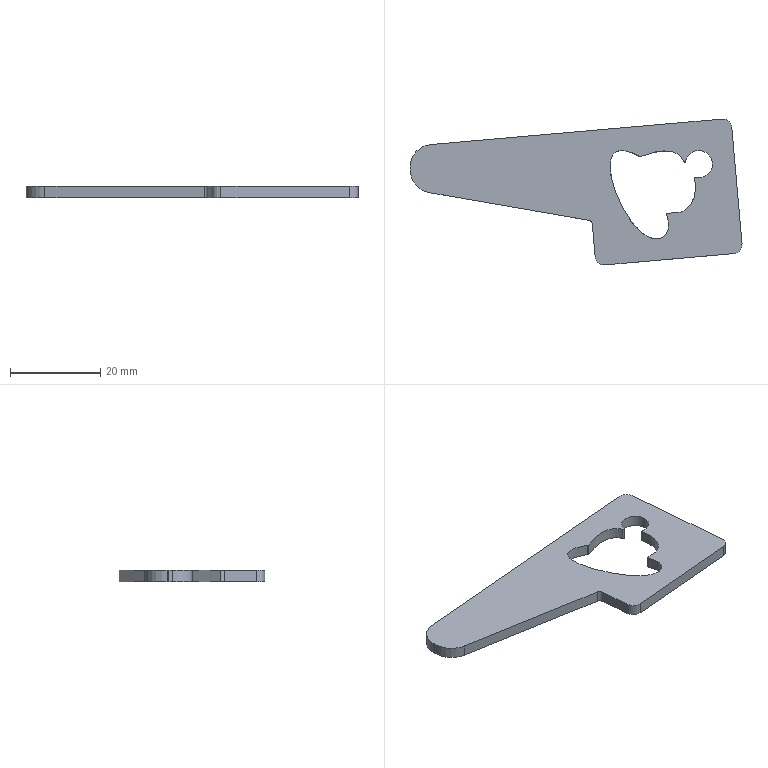Part | SolidWorks | features BaseBody 1 | 1 solid | 28 faces | box 73.757 x 32.407 x 2.5 mm | volume 3155 mm3 | cylinder 16 | plane 9 | spline 3 | commonest cylinder face diameters 0.4 x6 4 x3 6 x3 10 x3 2 x1
STEP:
#1=CARTESIAN_POINT('',(11.35,-18.25,15.));
#2=VERTEX_POINT('',#1);
#3=CARTESIAN_POINT('',(5.409,-17.656,15.));
#4=VERTEX_POINT('',#3);
#5=CARTESIAN_POINT('',(8.35,-18.25,15.));
#6=DIRECTION('',(0.,0.,1.));
#7=DIRECTION('',(1.,0.,0.));
#8=AXIS2_PLACEMENT_3D('',#5,#6,#7);
#9=CIRCLE('',#8,3.);
#10=EDGE_CURVE('',#2,#4,#9,.T.);
#11=ORIENTED_EDGE('',*,*,#10,.F.);
#12=CARTESIAN_POINT('',(11.35,-18.25,17.5));
#13=VERTEX_POINT('',#12);
#14=CARTESIAN_POINT('',(11.35,-18.25,15.));
#15=DIRECTION('',(0.,0.,1.));
#16=VECTOR('',#15,1000.);
#17=LINE('',#14,#16);
#18=EDGE_CURVE('',#2,#13,#17,.T.);
#19=ORIENTED_EDGE('',*,*,#18,.T.);
#20=CARTESIAN_POINT('',(5.409,-17.656,17.5));
#21=VERTEX_POINT('',#20);
#22=CARTESIAN_POINT('',(8.35,-18.25,17.5));
#23=DIRECTION('',(0.,0.,-1.));
#24=DIRECTION('',(1.,0.,0.));
#25=AXIS2_PLACEMENT_3D('',#22,#23,#24);
#26=CIRCLE('',#25,3.);
#27=EDGE_CURVE('',#21,#13,#26,.T.);
#28=ORIENTED_EDGE('',*,*,#27,.F.);
#29=CARTESIAN_POINT('',(5.409,-17.656,15.));
#30=DIRECTION('',(0.,0.,1.));
#31=VECTOR('',#30,1000.);
#32=LINE('',#29,#31);
#33=EDGE_CURVE('',#4,#21,#32,.T.);
#34=ORIENTED_EDGE('',*,*,#33,.F.);
#35=EDGE_LOOP('',(#11,#19,#28,#34));
#36=FACE_OUTER_BOUND('',#35,.T.);
#37=CARTESIAN_POINT('',(8.35,-18.25,15.));
#38=DIRECTION('',(0.,0.,1.));
#39=DIRECTION('',(1.,0.,0.));
#40=AXIS2_PLACEMENT_3D('',#37,#38,#39);
#41=CYLINDRICAL_SURFACE('',#40,3.);
#42=ADVANCED_FACE('',(#36),#41,.F.);
#43=CARTESIAN_POINT('',(-55.818,-18.909,17.5));
#44=VERTEX_POINT('',#43);
#45=CARTESIAN_POINT('',(-55.799,-19.345,17.5));
#46=VERTEX_POINT('',#45);
#47=CARTESIAN_POINT('',(-50.818,-18.909,17.5));
#48=DIRECTION('',(0.,0.,1.));
#49=DIRECTION('',(-1.,0.,0.));
#50=AXIS2_PLACEMENT_3D('',#47,#48,#49);
#51=CIRCLE('',#50,5.);
#52=EDGE_CURVE('',#44,#46,#51,.T.);
#53=ORIENTED_EDGE('',*,*,#52,.F.);
#54=CARTESIAN_POINT('',(-55.818,-18.909,15.));
#55=VERTEX_POINT('',#54);
#56=CARTESIAN_POINT('',(-55.818,-18.909,23.765));
#57=DIRECTION('',(0.,0.,-1.));
#58=VECTOR('',#57,1000.);
#59=LINE('',#56,#58);
#60=EDGE_CURVE('',#44,#55,#59,.T.);
#61=ORIENTED_EDGE('',*,*,#60,.T.);
#62=CARTESIAN_POINT('',(-55.799,-19.345,15.));
#63=VERTEX_POINT('',#62);
#64=CARTESIAN_POINT('',(-50.818,-18.909,15.));
#65=DIRECTION('',(0.,0.,1.));
#66=DIRECTION('',(-1.,0.,0.));
#67=AXIS2_PLACEMENT_3D('',#64,#65,#66);
#68=CIRCLE('',#67,5.);
#69=EDGE_CURVE('',#55,#63,#68,.T.);
#70=ORIENTED_EDGE('',*,*,#69,.T.);
#71=CARTESIAN_POINT('',(-55.799,-19.345,23.765));
#72=DIRECTION('',(0.,0.,1.));
#73=VECTOR('',#72,1000.);
#74=LINE('',#71,#73);
#75=EDGE_CURVE('',#63,#46,#74,.T.);
#76=ORIENTED_EDGE('',*,*,#75,.T.);
#77=EDGE_LOOP('',(#53,#61,#70,#76));
#78=FACE_OUTER_BOUND('',#77,.T.);
#79=CARTESIAN_POINT('',(-50.818,-18.909,23.765));
#80=DIRECTION('',(0.,0.,-1.));
#81=DIRECTION('',(-1.,0.,0.));
#82=AXIS2_PLACEMENT_3D('',#79,#80,#81);
#83=CYLINDRICAL_SURFACE('',#82,5.);
#84=ADVANCED_FACE('',(#78),#83,.T.);
#85=CARTESIAN_POINT('',(1.217,-29.458,17.5));
#86=VERTEX_POINT('',#85);
#87=CARTESIAN_POINT('',(1.208,-29.397,17.5));
#88=VERTEX_POINT('',#87);
#89=CARTESIAN_POINT('',(1.408,-29.397,17.5));
#90=DIRECTION('',(0.,0.,-1.));
#91=DIRECTION('',(-1.,0.,0.));
#92=AXIS2_PLACEMENT_3D('',#89,#90,#91);
#93=CIRCLE('',#92,0.2);
#94=EDGE_CURVE('',#86,#88,#93,.T.);
#95=ORIENTED_EDGE('',*,*,#94,.T.);
#96=CARTESIAN_POINT('',(1.208,-29.397,15.));
#97=VERTEX_POINT('',#96);
#98=CARTESIAN_POINT('',(1.208,-29.397,20.759));
#99=DIRECTION('',(0.,0.,-1.));
#100=VECTOR('',#99,1000.);
#101=LINE('',#98,#100);
#102=EDGE_CURVE('',#88,#97,#101,.T.);
#103=ORIENTED_EDGE('',*,*,#102,.T.);
#104=CARTESIAN_POINT('',(1.217,-29.458,15.));
#105=VERTEX_POINT('',#104);
#106=CARTESIAN_POINT('',(1.408,-29.397,15.));
#107=DIRECTION('',(0.,0.,1.));
#108=DIRECTION('',(-1.,0.,0.));
#109=AXIS2_PLACEMENT_3D('',#106,#107,#108);
#110=CIRCLE('',#109,0.2);
#111=EDGE_CURVE('',#97,#105,#110,.T.);
#112=ORIENTED_EDGE('',*,*,#111,.T.);
#113=CARTESIAN_POINT('',(1.217,-29.458,16.25));
#114=DIRECTION('',(0.,0.,1.));
#115=VECTOR('',#114,1000.);
#116=LINE('',#113,#115);
#117=EDGE_CURVE('',#105,#86,#116,.T.);
#118=ORIENTED_EDGE('',*,*,#117,.T.);
#119=EDGE_LOOP('',(#95,#103,#112,#118));
#120=FACE_OUTER_BOUND('',#119,.T.);
#121=CARTESIAN_POINT('',(1.408,-29.397,20.759));
#122=DIRECTION('',(0.,0.,-1.));
#123=DIRECTION('',(-1.,0.,0.));
#124=AXIS2_PLACEMENT_3D('',#121,#122,#123);
#125=CYLINDRICAL_SURFACE('',#124,0.2);
#126=ADVANCED_FACE('',(#120),#125,.T.);
#127=CARTESIAN_POINT('',(7.403,-21.403,17.5));
#128=VERTEX_POINT('',#127);
#129=CARTESIAN_POINT('',(7.398,-21.36,17.5));
#130=VERTEX_POINT('',#129);
#131=CARTESIAN_POINT('',(7.598,-21.36,17.5));
#132=DIRECTION('',(0.,0.,-1.));
#133=DIRECTION('',(-1.,0.,0.));
#134=AXIS2_PLACEMENT_3D('',#131,#132,#133);
#135=CIRCLE('',#134,0.2);
#136=EDGE_CURVE('',#128,#130,#135,.T.);
#137=ORIENTED_EDGE('',*,*,#136,.T.);
#138=CARTESIAN_POINT('',(7.398,-21.36,15.));
#139=VERTEX_POINT('',#138);
#140=CARTESIAN_POINT('',(7.398,-21.36,20.759));
#141=DIRECTION('',(0.,0.,-1.));
#142=VECTOR('',#141,1000.);
#143=LINE('',#140,#142);
#144=EDGE_CURVE('',#130,#139,#143,.T.);
#145=ORIENTED_EDGE('',*,*,#144,.T.);
#146=CARTESIAN_POINT('',(7.403,-21.403,15.));
#147=VERTEX_POINT('',#146);
#148=CARTESIAN_POINT('',(7.598,-21.36,15.));
#149=DIRECTION('',(0.,0.,1.));
#150=DIRECTION('',(-1.,0.,0.));
#151=AXIS2_PLACEMENT_3D('',#148,#149,#150);
#152=CIRCLE('',#151,0.2);
#153=EDGE_CURVE('',#139,#147,#152,.T.);
#154=ORIENTED_EDGE('',*,*,#153,.T.);
#155=CARTESIAN_POINT('',(7.403,-21.403,16.25));
#156=DIRECTION('',(0.,0.,1.));
#157=VECTOR('',#156,1000.);
#158=LINE('',#155,#157);
#159=EDGE_CURVE('',#147,#128,#158,.T.);
#160=ORIENTED_EDGE('',*,*,#159,.T.);
#161=EDGE_LOOP('',(#137,#145,#154,#160));
#162=FACE_OUTER_BOUND('',#161,.T.);
#163=CARTESIAN_POINT('',(7.598,-21.36,20.759));
#164=DIRECTION('',(0.,0.,-1.));
#165=DIRECTION('',(-1.,0.,0.));
#166=AXIS2_PLACEMENT_3D('',#163,#164,#165);
#167=CYLINDRICAL_SURFACE('',#166,0.2);
#168=ADVANCED_FACE('',(#162),#167,.T.);
#169=CARTESIAN_POINT('',(5.629,-28.182,17.5));
#170=VERTEX_POINT('',#169);
#171=CARTESIAN_POINT('',(3.837,-28.984,17.5));
#172=VERTEX_POINT('',#171);
#173=CARTESIAN_POINT('',(3.575,-25.996,17.5));
#174=DIRECTION('',(0.,0.,-1.));
#175=DIRECTION('',(1.,0.,0.));
#176=AXIS2_PLACEMENT_3D('',#173,#174,#175);
#177=CIRCLE('',#176,3.);
#178=EDGE_CURVE('',#170,#172,#177,.T.);
#179=ORIENTED_EDGE('',*,*,#178,.T.);
#180=CARTESIAN_POINT('',(1.39,-29.198,17.5));
#181=VERTEX_POINT('',#180);
#182=CARTESIAN_POINT('',(3.837,-28.984,17.5));
#183=DIRECTION('',(-0.9962,-0.08716,0.));
#184=VECTOR('',#183,1000.);
#185=LINE('',#182,#184);
#186=EDGE_CURVE('',#172,#181,#185,.T.);
#187=ORIENTED_EDGE('',*,*,#186,.T.);
#188=CARTESIAN_POINT('',(1.408,-29.397,17.5));
#189=DIRECTION('',(0.,0.,-1.));
#190=DIRECTION('',(-1.,0.,0.));
#191=AXIS2_PLACEMENT_3D('',#188,#189,#190);
#192=CIRCLE('',#191,0.2);
#193=EDGE_CURVE('',#88,#181,#192,.T.);
#194=ORIENTED_EDGE('',*,*,#193,.F.);
#195=ORIENTED_EDGE('',*,*,#94,.F.);
#196=CARTESIAN_POINT('',(-4.863,-16.57,17.5));
#197=VERTEX_POINT('',#196);
#198=CARTESIAN_POINT('',(1.217,-29.458,17.5));
#199=CARTESIAN_POINT('',(2.365,-33.062,17.5));
#200=CARTESIAN_POINT('',(-1.868,-37.339,17.5));
#201=CARTESIAN_POINT('',(-10.191,-27.786,17.5));
#202=CARTESIAN_POINT('',(-12.869,-14.51,17.5));
#203=CARTESIAN_POINT('',(-7.281,-15.123,17.5));
#204=CARTESIAN_POINT('',(-4.863,-16.57,17.5));
#205=B_SPLINE_CURVE_WITH_KNOTS('',3,(#198,#199,#200,#201,#202,#203,#204),.UNSPECIFIED.,.F.,.F.,(4,1,1,1,4),(0.,0.006113,0.01872,0.03058,0.03634),.UNSPECIFIED.);
#206=EDGE_CURVE('',#86,#197,#205,.T.);
#207=ORIENTED_EDGE('',*,*,#206,.T.);
#208=CARTESIAN_POINT('',(-4.693,-16.587,17.5));
#209=VERTEX_POINT('',#208);
#210=CARTESIAN_POINT('',(-4.76,-16.398,17.5));
#211=DIRECTION('',(0.,0.,-1.));
#212=DIRECTION('',(-1.,0.,0.));
#213=AXIS2_PLACEMENT_3D('',#210,#211,#212);
#214=CIRCLE('',#213,0.2);
#215=EDGE_CURVE('',#209,#197,#214,.T.);
#216=ORIENTED_EDGE('',*,*,#215,.F.);
#217=CARTESIAN_POINT('',(5.033,-17.703,17.5));
#218=VERTEX_POINT('',#217);
#219=CARTESIAN_POINT('',(-4.693,-16.587,17.5));
#220=CARTESIAN_POINT('',(-1.674,-15.514,17.5));
#221=CARTESIAN_POINT('',(2.462,-14.423,17.5));
#222=CARTESIAN_POINT('',(4.678,-16.963,17.5));
#223=CARTESIAN_POINT('',(5.033,-17.703,17.5));
#224=B_SPLINE_CURVE_WITH_KNOTS('',3,(#219,#220,#221,#222,#223),.UNSPECIFIED.,.F.,.F.,(4,1,4),(0.,0.008476,0.01075),.UNSPECIFIED.);
#225=EDGE_CURVE('',#209,#218,#224,.T.);
#226=ORIENTED_EDGE('',*,*,#225,.T.);
#227=CARTESIAN_POINT('',(5.213,-17.617,17.5));
#228=DIRECTION('',(0.,0.,-1.));
#229=DIRECTION('',(-1.,0.,0.));
#230=AXIS2_PLACEMENT_3D('',#227,#228,#229);
#231=CIRCLE('',#230,0.2);
#232=EDGE_CURVE('',#21,#218,#231,.T.);
#233=ORIENTED_EDGE('',*,*,#232,.F.);
#234=ORIENTED_EDGE('',*,*,#27,.T.);
#235=CARTESIAN_POINT('',(7.645,-21.166,17.5));
#236=VERTEX_POINT('',#235);
#237=CARTESIAN_POINT('',(8.35,-18.25,17.5));
#238=DIRECTION('',(0.,0.,-1.));
#239=DIRECTION('',(1.,0.,0.));
#240=AXIS2_PLACEMENT_3D('',#237,#238,#239);
#241=CIRCLE('',#240,3.);
#242=EDGE_CURVE('',#13,#236,#241,.T.);
#243=ORIENTED_EDGE('',*,*,#242,.T.);
#244=CARTESIAN_POINT('',(7.598,-21.36,17.5));
#245=DIRECTION('',(0.,0.,-1.));
#246=DIRECTION('',(-1.,0.,0.));
#247=AXIS2_PLACEMENT_3D('',#244,#245,#246);
#248=CIRCLE('',#247,0.2);
#249=EDGE_CURVE('',#130,#236,#248,.T.);
#250=ORIENTED_EDGE('',*,*,#249,.F.);
#251=ORIENTED_EDGE('',*,*,#136,.F.);
#252=CARTESIAN_POINT('',(7.403,-21.403,17.5));
#253=CARTESIAN_POINT('',(8.013,-24.239,17.5));
#254=CARTESIAN_POINT('',(7.422,-26.499,17.5));
#255=CARTESIAN_POINT('',(5.629,-28.182,17.5));
#256=B_SPLINE_CURVE_WITH_KNOTS('',3,(#252,#253,#254,#255),.UNSPECIFIED.,.F.,.F.,(4,4),(0.,1.),.UNSPECIFIED.);
#257=EDGE_CURVE('',#128,#170,#256,.T.);
#258=ORIENTED_EDGE('',*,*,#257,.T.);
#259=EDGE_LOOP('',(#179,#187,#194,#195,#207,#216,#226,#233,#234,#243,#250,#251,#258));
#260=FACE_BOUND('',#259,.T.);
#261=CARTESIAN_POINT('',(-12.527,-40.655,17.5));
#262=VERTEX_POINT('',#261);
#263=CARTESIAN_POINT('',(16.114,-38.149,17.5));
#264=VERTEX_POINT('',#263);
#265=CARTESIAN_POINT('',(-12.527,-40.655,17.5));
#266=DIRECTION('',(0.9962,0.08716,0.));
#267=VECTOR('',#266,1000.);
#268=LINE('',#265,#267);
#269=EDGE_CURVE('',#262,#264,#268,.T.);
#270=ORIENTED_EDGE('',*,*,#269,.T.);
#271=CARTESIAN_POINT('',(17.932,-35.982,17.5));
#272=VERTEX_POINT('',#271);
#273=CARTESIAN_POINT('',(15.94,-36.157,17.5));
#274=DIRECTION('',(0.,0.,1.));
#275=DIRECTION('',(-1.,0.,0.));
#276=AXIS2_PLACEMENT_3D('',#273,#274,#275);
#277=CIRCLE('',#276,2.);
#278=EDGE_CURVE('',#264,#272,#277,.T.);
#279=ORIENTED_EDGE('',*,*,#278,.T.);
#280=CARTESIAN_POINT('',(15.666,-10.081,17.5));
#281=VERTEX_POINT('',#280);
#282=CARTESIAN_POINT('',(17.932,-35.982,17.5));
#283=DIRECTION('',(-0.08716,0.9962,0.));
#284=VECTOR('',#283,1000.);
#285=LINE('',#282,#284);
#286=EDGE_CURVE('',#272,#281,#285,.T.);
#287=ORIENTED_EDGE('',*,*,#286,.T.);
#288=CARTESIAN_POINT('',(13.499,-8.263,17.5));
#289=VERTEX_POINT('',#288);
#290=CARTESIAN_POINT('',(13.674,-10.256,17.5));
#291=DIRECTION('',(0.,0.,1.));
#292=DIRECTION('',(-1.,0.,0.));
#293=AXIS2_PLACEMENT_3D('',#290,#291,#292);
#294=CIRCLE('',#293,2.);
#295=EDGE_CURVE('',#281,#289,#294,.T.);
#296=ORIENTED_EDGE('',*,*,#295,.T.);
#297=CARTESIAN_POINT('',(-51.253,-13.928,17.5));
#298=VERTEX_POINT('',#297);
#299=CARTESIAN_POINT('',(13.499,-8.263,17.5));
#300=DIRECTION('',(-0.9962,-0.08716,0.));
#301=VECTOR('',#300,1000.);
#302=LINE('',#299,#301);
#303=EDGE_CURVE('',#289,#298,#302,.T.);
#304=ORIENTED_EDGE('',*,*,#303,.T.);
#305=CARTESIAN_POINT('',(-50.818,-18.909,17.5));
#306=DIRECTION('',(0.,0.,1.));
#307=DIRECTION('',(-1.,0.,0.));
#308=AXIS2_PLACEMENT_3D('',#305,#306,#307);
#309=CIRCLE('',#308,5.);
#310=EDGE_CURVE('',#298,#44,#309,.T.);
#311=ORIENTED_EDGE('',*,*,#310,.T.);
#312=ORIENTED_EDGE('',*,*,#52,.T.);
#313=CARTESIAN_POINT('',(-55.733,-20.095,17.5));
#314=VERTEX_POINT('',#313);
#315=CARTESIAN_POINT('',(-56.234,-14.364,17.5));
#316=DIRECTION('',(-0.08716,0.9962,0.));
#317=VECTOR('',#316,1000.);
#318=LINE('',#315,#317);
#319=EDGE_CURVE('',#314,#46,#318,.T.);
#320=ORIENTED_EDGE('',*,*,#319,.F.);
#321=CARTESIAN_POINT('',(-51.607,-24.585,17.5));
#322=VERTEX_POINT('',#321);
#323=CARTESIAN_POINT('',(-50.752,-19.659,17.5));
#324=DIRECTION('',(0.,0.,1.));
#325=DIRECTION('',(-1.,0.,0.));
#326=AXIS2_PLACEMENT_3D('',#323,#324,#325);
#327=CIRCLE('',#326,5.);
#328=EDGE_CURVE('',#314,#322,#327,.T.);
#329=ORIENTED_EDGE('',*,*,#328,.T.);
#330=CARTESIAN_POINT('',(-16.149,-30.736,17.5));
#331=VERTEX_POINT('',#330);
#332=CARTESIAN_POINT('',(-51.607,-24.585,17.5));
#333=DIRECTION('',(0.9853,-0.1709,0.));
#334=VECTOR('',#333,1000.);
#335=LINE('',#332,#334);
#336=EDGE_CURVE('',#322,#331,#335,.T.);
#337=ORIENTED_EDGE('',*,*,#336,.T.);
#338=CARTESIAN_POINT('',(-15.324,-31.634,17.5));
#339=VERTEX_POINT('',#338);
#340=CARTESIAN_POINT('',(-16.32,-31.721,17.5));
#341=DIRECTION('',(0.,0.,-1.));
#342=DIRECTION('',(1.,0.,0.));
#343=AXIS2_PLACEMENT_3D('',#340,#341,#342);
#344=CIRCLE('',#343,1.);
#345=EDGE_CURVE('',#331,#339,#344,.T.);
#346=ORIENTED_EDGE('',*,*,#345,.T.);
#347=CARTESIAN_POINT('',(-14.693,-38.837,17.5));
#348=VERTEX_POINT('',#347);
#349=CARTESIAN_POINT('',(-15.324,-31.634,17.5));
#350=DIRECTION('',(0.08716,-0.9962,0.));
#351=VECTOR('',#350,1000.);
#352=LINE('',#349,#351);
#353=EDGE_CURVE('',#339,#348,#352,.T.);
#354=ORIENTED_EDGE('',*,*,#353,.T.);
#355=CARTESIAN_POINT('',(-12.701,-38.662,17.5));
#356=DIRECTION('',(0.,0.,1.));
#357=DIRECTION('',(-1.,0.,0.));
#358=AXIS2_PLACEMENT_3D('',#355,#356,#357);
#359=CIRCLE('',#358,2.);
#360=EDGE_CURVE('',#348,#262,#359,.T.);
#361=ORIENTED_EDGE('',*,*,#360,.T.);
#362=EDGE_LOOP('',(#270,#279,#287,#296,#304,#311,#312,#320,#329,#337,#346,#354,#361));
#363=FACE_OUTER_BOUND('',#362,.T.);
#364=CARTESIAN_POINT('',(15.492,-8.089,17.5));
#365=DIRECTION('',(0.,0.,1.));
#366=DIRECTION('',(1.,0.,0.));
#367=AXIS2_PLACEMENT_3D('',#364,#365,#366);
#368=PLANE('',#367);
#369=ADVANCED_FACE('',(#260,#363),#368,.T.);
#370=ORIENTED_EDGE('',*,*,#186,.F.);
#371=CARTESIAN_POINT('',(3.837,-28.984,15.));
#372=VERTEX_POINT('',#371);
#373=CARTESIAN_POINT('',(3.837,-28.984,15.));
#374=DIRECTION('',(0.,0.,-1.));
#375=VECTOR('',#374,1000.);
#376=LINE('',#373,#375);
#377=EDGE_CURVE('',#172,#372,#376,.T.);
#378=ORIENTED_EDGE('',*,*,#377,.T.);
#379=CARTESIAN_POINT('',(1.39,-29.198,15.));
#380=VERTEX_POINT('',#379);
#381=CARTESIAN_POINT('',(4.735,-28.906,15.));
#382=DIRECTION('',(-0.9962,-0.08716,0.));
#383=VECTOR('',#382,1000.);
#384=LINE('',#381,#383);
#385=EDGE_CURVE('',#372,#380,#384,.T.);
#386=ORIENTED_EDGE('',*,*,#385,.T.);
#387=CARTESIAN_POINT('',(1.39,-29.198,15.));
#388=DIRECTION('',(0.,0.,1.));
#389=VECTOR('',#388,1000.);
#390=LINE('',#387,#389);
#391=EDGE_CURVE('',#380,#181,#390,.T.);
#392=ORIENTED_EDGE('',*,*,#391,.T.);
#393=EDGE_LOOP('',(#370,#378,#386,#392));
#394=FACE_OUTER_BOUND('',#393,.T.);
#395=CARTESIAN_POINT('',(4.735,-28.906,15.));
#396=DIRECTION('',(-0.08716,0.9962,0.));
#397=DIRECTION('',(-0.9962,-0.08716,0.));
#398=AXIS2_PLACEMENT_3D('',#395,#396,#397);
#399=PLANE('',#398);
#400=ADVANCED_FACE('',(#394),#399,.T.);
#401=CARTESIAN_POINT('',(5.629,-28.182,15.));
#402=VERTEX_POINT('',#401);
#403=CARTESIAN_POINT('',(5.629,-28.182,11.14));
#404=DIRECTION('',(0.,0.,1.));
#405=VECTOR('',#404,1000.);
#406=LINE('',#403,#405);
#407=EDGE_CURVE('',#402,#170,#406,.T.);
#408=ORIENTED_EDGE('',*,*,#407,.F.);
#409=CARTESIAN_POINT('',(3.575,-25.996,15.));
#410=DIRECTION('',(0.,0.,1.));
#411=DIRECTION('',(1.,0.,0.));
#412=AXIS2_PLACEMENT_3D('',#409,#410,#411);
#413=CIRCLE('',#412,3.);
#414=EDGE_CURVE('',#372,#402,#413,.T.);
#415=ORIENTED_EDGE('',*,*,#414,.F.);
#416=ORIENTED_EDGE('',*,*,#377,.F.);
#417=ORIENTED_EDGE('',*,*,#178,.F.);
#418=EDGE_LOOP('',(#408,#415,#416,#417));
#419=FACE_OUTER_BOUND('',#418,.T.);
#420=CARTESIAN_POINT('',(3.575,-25.996,11.14));
#421=DIRECTION('',(0.,0.,1.));
#422=DIRECTION('',(1.,0.,0.));
#423=AXIS2_PLACEMENT_3D('',#420,#421,#422);
#424=CYLINDRICAL_SURFACE('',#423,3.);
#425=ADVANCED_FACE('',(#419),#424,.F.);
#426=ORIENTED_EDGE('',*,*,#159,.F.);
#427=CARTESIAN_POINT('',(5.629,-28.182,15.));
#428=CARTESIAN_POINT('',(7.422,-26.499,15.));
#429=CARTESIAN_POINT('',(8.013,-24.239,15.));
#430=CARTESIAN_POINT('',(7.403,-21.403,15.));
#431=B_SPLINE_CURVE_WITH_KNOTS('',3,(#427,#428,#429,#430),.UNSPECIFIED.,.F.,.F.,(4,4),(0.,1.),.UNSPECIFIED.);
#432=EDGE_CURVE('',#402,#147,#431,.T.);
#433=ORIENTED_EDGE('',*,*,#432,.F.);
#434=ORIENTED_EDGE('',*,*,#407,.T.);
#435=ORIENTED_EDGE('',*,*,#257,.F.);
#436=EDGE_LOOP('',(#426,#433,#434,#435));
#437=FACE_OUTER_BOUND('',#436,.T.);
#438=CARTESIAN_POINT('',(5.629,-28.182,15.));
#439=CARTESIAN_POINT('',(5.629,-28.182,17.5));
#440=CARTESIAN_POINT('',(6.029,-27.807,15.));
#441=CARTESIAN_POINT('',(6.029,-27.807,17.5));
#442=CARTESIAN_POINT('',(7.554,-25.995,15.));
#443=CARTESIAN_POINT('',(7.554,-25.995,17.5));
#444=CARTESIAN_POINT('',(7.877,-23.607,15.));
#445=CARTESIAN_POINT('',(7.877,-23.607,17.5));
#446=CARTESIAN_POINT('',(7.403,-21.403,15.));
#447=CARTESIAN_POINT('',(7.403,-21.403,17.5));
#448=B_SPLINE_SURFACE_WITH_KNOTS('',3,1,((#438,#439),(#440,#441),(#442,#443),(#444,#445),(#446,#447)),.UNSPECIFIED.,.F.,.F.,.F.,(4,1,4),(2,2),(0.009234,0.2282,0.9918),(0.,1.),.UNSPECIFIED.);
#449=ADVANCED_FACE('',(#437),#448,.F.);
#450=ORIENTED_EDGE('',*,*,#18,.F.);
#451=CARTESIAN_POINT('',(7.645,-21.166,15.));
#452=VERTEX_POINT('',#451);
#453=CARTESIAN_POINT('',(8.35,-18.25,15.));
#454=DIRECTION('',(0.,0.,1.));
#455=DIRECTION('',(1.,0.,0.));
#456=AXIS2_PLACEMENT_3D('',#453,#454,#455);
#457=CIRCLE('',#456,3.);
#458=EDGE_CURVE('',#452,#2,#457,.T.);
#459=ORIENTED_EDGE('',*,*,#458,.F.);
#460=CARTESIAN_POINT('',(7.645,-21.166,15.));
#461=DIRECTION('',(0.,0.,-1.));
#462=VECTOR('',#461,1000.);
#463=LINE('',#460,#462);
#464=EDGE_CURVE('',#236,#452,#463,.T.);
#465=ORIENTED_EDGE('',*,*,#464,.F.);
#466=ORIENTED_EDGE('',*,*,#242,.F.);
#467=EDGE_LOOP('',(#450,#459,#465,#466));
#468=FACE_OUTER_BOUND('',#467,.T.);
#469=CARTESIAN_POINT('',(8.35,-18.25,15.));
#470=DIRECTION('',(0.,0.,1.));
#471=DIRECTION('',(1.,0.,0.));
#472=AXIS2_PLACEMENT_3D('',#469,#470,#471);
#473=CYLINDRICAL_SURFACE('',#472,3.);
#474=ADVANCED_FACE('',(#468),#473,.F.);
#475=CARTESIAN_POINT('',(-4.693,-16.587,15.));
#476=VERTEX_POINT('',#475);
#477=CARTESIAN_POINT('',(-4.693,-16.587,16.25));
#478=DIRECTION('',(0.,0.,1.));
#479=VECTOR('',#478,1000.);
#480=LINE('',#477,#479);
#481=EDGE_CURVE('',#476,#209,#480,.T.);
#482=ORIENTED_EDGE('',*,*,#481,.F.);
#483=CARTESIAN_POINT('',(5.033,-17.703,15.));
#484=VERTEX_POINT('',#483);
#485=CARTESIAN_POINT('',(5.033,-17.703,15.));
#486=CARTESIAN_POINT('',(4.678,-16.963,15.));
#487=CARTESIAN_POINT('',(2.462,-14.423,15.));
#488=CARTESIAN_POINT('',(-1.674,-15.514,15.));
#489=CARTESIAN_POINT('',(-4.693,-16.587,15.));
#490=B_SPLINE_CURVE_WITH_KNOTS('',3,(#485,#486,#487,#488,#489),.UNSPECIFIED.,.F.,.F.,(4,1,4),(0.,0.002298,0.01085),.UNSPECIFIED.);
#491=EDGE_CURVE('',#484,#476,#490,.T.);
#492=ORIENTED_EDGE('',*,*,#491,.F.);
#493=CARTESIAN_POINT('',(5.033,-17.703,16.25));
#494=DIRECTION('',(0.,0.,-1.));
#495=VECTOR('',#494,1000.);
#496=LINE('',#493,#495);
#497=EDGE_CURVE('',#218,#484,#496,.T.);
#498=ORIENTED_EDGE('',*,*,#497,.F.);
#499=ORIENTED_EDGE('',*,*,#225,.F.);
#500=EDGE_LOOP('',(#482,#492,#498,#499));
#501=FACE_OUTER_BOUND('',#500,.T.);
#502=CARTESIAN_POINT('',(5.033,-17.703,15.));
#503=CARTESIAN_POINT('',(5.033,-17.703,17.5));
#504=CARTESIAN_POINT('',(4.678,-16.963,15.));
#505=CARTESIAN_POINT('',(4.678,-16.963,17.5));
#506=CARTESIAN_POINT('',(2.462,-14.423,15.));
#507=CARTESIAN_POINT('',(2.462,-14.423,17.5));
#508=CARTESIAN_POINT('',(-1.674,-15.514,15.));
#509=CARTESIAN_POINT('',(-1.674,-15.514,17.5));
#510=CARTESIAN_POINT('',(-4.693,-16.587,15.));
#511=CARTESIAN_POINT('',(-4.693,-16.587,17.5));
#512=B_SPLINE_SURFACE_WITH_KNOTS('',3,1,((#502,#503),(#504,#505),(#506,#507),(#508,#509),(#510,#511)),.UNSPECIFIED.,.F.,.F.,.F.,(4,1,4),(2,2),(0.00811,0.2164,0.9912),(0.,1.),.UNSPECIFIED.);
#513=ADVANCED_FACE('',(#501),#512,.F.);
#514=ORIENTED_EDGE('',*,*,#117,.F.);
#515=CARTESIAN_POINT('',(-4.863,-16.57,15.));
#516=VERTEX_POINT('',#515);
#517=CARTESIAN_POINT('',(-4.863,-16.57,15.));
#518=CARTESIAN_POINT('',(-7.281,-15.123,15.));
#519=CARTESIAN_POINT('',(-12.869,-14.51,15.));
#520=CARTESIAN_POINT('',(-10.191,-27.786,15.));
#521=CARTESIAN_POINT('',(-1.868,-37.339,15.));
#522=CARTESIAN_POINT('',(2.365,-33.062,15.));
#523=CARTESIAN_POINT('',(1.217,-29.458,15.));
#524=B_SPLINE_CURVE_WITH_KNOTS('',3,(#517,#518,#519,#520,#521,#522,#523),.UNSPECIFIED.,.F.,.F.,(4,1,1,1,4),(0.,0.005774,0.01766,0.03028,0.03641),.UNSPECIFIED.);
#525=EDGE_CURVE('',#516,#105,#524,.T.);
#526=ORIENTED_EDGE('',*,*,#525,.F.);
#527=CARTESIAN_POINT('',(-4.863,-16.57,16.25));
#528=DIRECTION('',(0.,0.,-1.));
#529=VECTOR('',#528,1000.);
#530=LINE('',#527,#529);
#531=EDGE_CURVE('',#197,#516,#530,.T.);
#532=ORIENTED_EDGE('',*,*,#531,.F.);
#533=ORIENTED_EDGE('',*,*,#206,.F.);
#534=EDGE_LOOP('',(#514,#526,#532,#533));
#535=FACE_OUTER_BOUND('',#534,.T.);
#536=CARTESIAN_POINT('',(-4.863,-16.57,15.));
#537=CARTESIAN_POINT('',(-4.863,-16.57,17.5));
#538=CARTESIAN_POINT('',(-7.281,-15.123,15.));
#539=CARTESIAN_POINT('',(-7.281,-15.123,17.5));
#540=CARTESIAN_POINT('',(-12.869,-14.51,15.));
#541=CARTESIAN_POINT('',(-12.869,-14.51,17.5));
#542=CARTESIAN_POINT('',(-10.191,-27.786,15.));
#543=CARTESIAN_POINT('',(-10.191,-27.786,17.5));
#544=CARTESIAN_POINT('',(-1.868,-37.339,15.));
#545=CARTESIAN_POINT('',(-1.868,-37.339,17.5));
#546=CARTESIAN_POINT('',(2.365,-33.062,15.));
#547=CARTESIAN_POINT('',(2.365,-33.062,17.5));
#548=CARTESIAN_POINT('',(1.217,-29.458,15.));
#549=CARTESIAN_POINT('',(1.217,-29.458,17.5));
#550=B_SPLINE_SURFACE_WITH_KNOTS('',3,1,((#536,#537),(#538,#539),(#540,#541),(#542,#543),(#544,#545),(#546,#547),(#548,#549)),.UNSPECIFIED.,.F.,.F.,.F.,(4,1,1,1,4),(2,2),(0.006613,0.1633,0.4858,0.8285,0.9947),(0.,1.),.UNSPECIFIED.);
#551=ADVANCED_FACE('',(#535),#550,.F.);
#552=CARTESIAN_POINT('',(16.114,-38.149,15.));
#553=VERTEX_POINT('',#552);
#554=CARTESIAN_POINT('',(16.114,-38.149,20.759));
#555=DIRECTION('',(0.,0.,-1.));
#556=VECTOR('',#555,1000.);
#557=LINE('',#554,#556);
#558=EDGE_CURVE('',#264,#553,#557,.T.);
#559=ORIENTED_EDGE('',*,*,#558,.T.);
#560=CARTESIAN_POINT('',(17.932,-35.982,15.));
#561=VERTEX_POINT('',#560);
#562=CARTESIAN_POINT('',(15.94,-36.157,15.));
#563=DIRECTION('',(0.,0.,1.));
#564=DIRECTION('',(-1.,0.,0.));
#565=AXIS2_PLACEMENT_3D('',#562,#563,#564);
#566=CIRCLE('',#565,2.);
#567=EDGE_CURVE('',#553,#561,#566,.T.);
#568=ORIENTED_EDGE('',*,*,#567,.T.);
#569=CARTESIAN_POINT('',(17.932,-35.982,20.759));
#570=DIRECTION('',(0.,0.,1.));
#571=VECTOR('',#570,1000.);
#572=LINE('',#569,#571);
#573=EDGE_CURVE('',#561,#272,#572,.T.);
#574=ORIENTED_EDGE('',*,*,#573,.T.);
#575=ORIENTED_EDGE('',*,*,#278,.F.);
#576=EDGE_LOOP('',(#559,#568,#574,#575));
#577=FACE_OUTER_BOUND('',#576,.T.);
#578=CARTESIAN_POINT('',(15.94,-36.157,20.759));
#579=DIRECTION('',(0.,0.,-1.));
#580=DIRECTION('',(-1.,0.,0.));
#581=AXIS2_PLACEMENT_3D('',#578,#579,#580);
#582=CYLINDRICAL_SURFACE('',#581,2.);
#583=ADVANCED_FACE('',(#577),#582,.T.);
#584=CARTESIAN_POINT('',(-12.527,-40.655,15.));
#585=VERTEX_POINT('',#584);
#586=CARTESIAN_POINT('',(-14.519,-40.829,15.));
#587=DIRECTION('',(0.9962,0.08716,0.));
#588=VECTOR('',#587,1000.);
#589=LINE('',#586,#588);
#590=EDGE_CURVE('',#585,#553,#589,.T.);
#591=ORIENTED_EDGE('',*,*,#590,.T.);
#592=ORIENTED_EDGE('',*,*,#558,.F.);
#593=ORIENTED_EDGE('',*,*,#269,.F.);
#594=CARTESIAN_POINT('',(-12.527,-40.655,15.));
#595=DIRECTION('',(0.,0.,-1.));
#596=VECTOR('',#595,1000.);
#597=LINE('',#594,#596);
#598=EDGE_CURVE('',#262,#585,#597,.T.);
#599=ORIENTED_EDGE('',*,*,#598,.T.);
#600=EDGE_LOOP('',(#591,#592,#593,#599));
#601=FACE_OUTER_BOUND('',#600,.T.);
#602=CARTESIAN_POINT('',(-14.519,-40.829,15.));
#603=DIRECTION('',(0.08716,-0.9962,0.));
#604=DIRECTION('',(0.9962,0.08716,0.));
#605=AXIS2_PLACEMENT_3D('',#602,#603,#604);
#606=PLANE('',#605);
#607=ADVANCED_FACE('',(#601),#606,.T.);
#608=CARTESIAN_POINT('',(-14.693,-38.837,15.));
#609=VERTEX_POINT('',#608);
#610=CARTESIAN_POINT('',(-14.693,-38.837,20.759));
#611=DIRECTION('',(0.,0.,-1.));
#612=VECTOR('',#611,1000.);
#613=LINE('',#610,#612);
#614=EDGE_CURVE('',#348,#609,#613,.T.);
#615=ORIENTED_EDGE('',*,*,#614,.T.);
#616=CARTESIAN_POINT('',(-12.701,-38.662,15.));
#617=DIRECTION('',(0.,0.,1.));
#618=DIRECTION('',(-1.,0.,0.));
#619=AXIS2_PLACEMENT_3D('',#616,#617,#618);
#620=CIRCLE('',#619,2.);
#621=EDGE_CURVE('',#609,#585,#620,.T.);
#622=ORIENTED_EDGE('',*,*,#621,.T.);
#623=ORIENTED_EDGE('',*,*,#598,.F.);
#624=ORIENTED_EDGE('',*,*,#360,.F.);
#625=EDGE_LOOP('',(#615,#622,#623,#624));
#626=FACE_OUTER_BOUND('',#625,.T.);
#627=CARTESIAN_POINT('',(-12.701,-38.662,20.759));
#628=DIRECTION('',(0.,0.,-1.));
#629=DIRECTION('',(-1.,0.,0.));
#630=AXIS2_PLACEMENT_3D('',#627,#628,#629);
#631=CYLINDRICAL_SURFACE('',#630,2.);
#632=ADVANCED_FACE('',(#626),#631,.T.);
#633=CARTESIAN_POINT('',(-15.324,-31.634,15.));
#634=VERTEX_POINT('',#633);
#635=CARTESIAN_POINT('',(-15.391,-30.867,15.));
#636=DIRECTION('',(0.08716,-0.9962,0.));
#637=VECTOR('',#636,1000.);
#638=LINE('',#635,#637);
#639=EDGE_CURVE('',#634,#609,#638,.T.);
#640=ORIENTED_EDGE('',*,*,#639,.T.);
#641=ORIENTED_EDGE('',*,*,#614,.F.);
#642=ORIENTED_EDGE('',*,*,#353,.F.);
#643=CARTESIAN_POINT('',(-15.324,-31.634,15.));
#644=DIRECTION('',(0.,0.,-1.));
#645=VECTOR('',#644,1000.);
#646=LINE('',#643,#645);
#647=EDGE_CURVE('',#339,#634,#646,.T.);
#648=ORIENTED_EDGE('',*,*,#647,.T.);
#649=EDGE_LOOP('',(#640,#641,#642,#648));
#650=FACE_OUTER_BOUND('',#649,.T.);
#651=CARTESIAN_POINT('',(-15.391,-30.867,15.));
#652=DIRECTION('',(-0.9962,-0.08716,0.));
#653=DIRECTION('',(0.08716,-0.9962,0.));
#654=AXIS2_PLACEMENT_3D('',#651,#652,#653);
#655=PLANE('',#654);
#656=ADVANCED_FACE('',(#650),#655,.T.);
#657=ORIENTED_EDGE('',*,*,#336,.F.);
#658=CARTESIAN_POINT('',(-51.607,-24.585,15.));
#659=VERTEX_POINT('',#658);
#660=CARTESIAN_POINT('',(-51.607,-24.585,15.));
#661=DIRECTION('',(0.,0.,-1.));
#662=VECTOR('',#661,1000.);
#663=LINE('',#660,#662);
#664=EDGE_CURVE('',#322,#659,#663,.T.);
#665=ORIENTED_EDGE('',*,*,#664,.T.);
#666=CARTESIAN_POINT('',(-16.149,-30.736,15.));
#667=VERTEX_POINT('',#666);
#668=CARTESIAN_POINT('',(-55.398,-23.928,15.));
#669=DIRECTION('',(0.9853,-0.1709,0.));
#670=VECTOR('',#669,1000.);
#671=LINE('',#668,#670);
#672=EDGE_CURVE('',#659,#667,#671,.T.);
#673=ORIENTED_EDGE('',*,*,#672,.T.);
#674=CARTESIAN_POINT('',(-16.149,-30.736,15.));
#675=DIRECTION('',(0.,0.,1.));
#676=VECTOR('',#675,1000.);
#677=LINE('',#674,#676);
#678=EDGE_CURVE('',#667,#331,#677,.T.);
#679=ORIENTED_EDGE('',*,*,#678,.T.);
#680=EDGE_LOOP('',(#657,#665,#673,#679));
#681=FACE_OUTER_BOUND('',#680,.T.);
#682=CARTESIAN_POINT('',(-55.398,-23.928,15.));
#683=DIRECTION('',(-0.1709,-0.9853,0.));
#684=DIRECTION('',(0.9853,-0.1709,0.));
#685=AXIS2_PLACEMENT_3D('',#682,#683,#684);
#686=PLANE('',#685);
#687=ADVANCED_FACE('',(#681),#686,.T.);
#688=CARTESIAN_POINT('',(-55.733,-20.095,15.));
#689=VERTEX_POINT('',#688);
#690=CARTESIAN_POINT('',(-55.733,-20.095,23.765));
#691=DIRECTION('',(0.,0.,-1.));
#692=VECTOR('',#691,1000.);
#693=LINE('',#690,#692);
#694=EDGE_CURVE('',#314,#689,#693,.T.);
#695=ORIENTED_EDGE('',*,*,#694,.T.);
#696=CARTESIAN_POINT('',(-50.752,-19.659,15.));
#697=DIRECTION('',(0.,0.,1.));
#698=DIRECTION('',(-1.,0.,0.));
#699=AXIS2_PLACEMENT_3D('',#696,#697,#698);
#700=CIRCLE('',#699,5.);
#701=EDGE_CURVE('',#689,#659,#700,.T.);
#702=ORIENTED_EDGE('',*,*,#701,.T.);
#703=ORIENTED_EDGE('',*,*,#664,.F.);
#704=ORIENTED_EDGE('',*,*,#328,.F.);
#705=EDGE_LOOP('',(#695,#702,#703,#704));
#706=FACE_OUTER_BOUND('',#705,.T.);
#707=CARTESIAN_POINT('',(-50.752,-19.659,23.765));
#708=DIRECTION('',(0.,0.,-1.));
#709=DIRECTION('',(-1.,0.,0.));
#710=AXIS2_PLACEMENT_3D('',#707,#708,#709);
#711=CYLINDRICAL_SURFACE('',#710,5.);
#712=ADVANCED_FACE('',(#706),#711,.T.);
#713=ORIENTED_EDGE('',*,*,#60,.F.);
#714=ORIENTED_EDGE('',*,*,#310,.F.);
#715=CARTESIAN_POINT('',(-51.253,-13.928,15.));
#716=VERTEX_POINT('',#715);
#717=CARTESIAN_POINT('',(-51.253,-13.928,23.765));
#718=DIRECTION('',(0.,0.,-1.));
#719=VECTOR('',#718,1000.);
#720=LINE('',#717,#719);
#721=EDGE_CURVE('',#298,#716,#720,.T.);
#722=ORIENTED_EDGE('',*,*,#721,.T.);
#723=CARTESIAN_POINT('',(-50.818,-18.909,15.));
#724=DIRECTION('',(0.,0.,1.));
#725=DIRECTION('',(-1.,0.,0.));
#726=AXIS2_PLACEMENT_3D('',#723,#724,#725);
#727=CIRCLE('',#726,5.);
#728=EDGE_CURVE('',#716,#55,#727,.T.);
#729=ORIENTED_EDGE('',*,*,#728,.T.);
#730=EDGE_LOOP('',(#713,#714,#722,#729));
#731=FACE_OUTER_BOUND('',#730,.T.);
#732=CARTESIAN_POINT('',(-50.818,-18.909,23.765));
#733=DIRECTION('',(0.,0.,-1.));
#734=DIRECTION('',(-1.,0.,0.));
#735=AXIS2_PLACEMENT_3D('',#732,#733,#734);
#736=CYLINDRICAL_SURFACE('',#735,5.);
#737=ADVANCED_FACE('',(#731),#736,.T.);
#738=ORIENTED_EDGE('',*,*,#303,.F.);
#739=CARTESIAN_POINT('',(13.499,-8.263,15.));
#740=VERTEX_POINT('',#739);
#741=CARTESIAN_POINT('',(13.499,-8.263,15.));
#742=DIRECTION('',(0.,0.,-1.));
#743=VECTOR('',#742,1000.);
#744=LINE('',#741,#743);
#745=EDGE_CURVE('',#289,#740,#744,.T.);
#746=ORIENTED_EDGE('',*,*,#745,.T.);
#747=CARTESIAN_POINT('',(15.492,-8.089,15.));
#748=DIRECTION('',(-0.9962,-0.08716,0.));
#749=VECTOR('',#748,1000.);
#750=LINE('',#747,#749);
#751=EDGE_CURVE('',#740,#716,#750,.T.);
#752=ORIENTED_EDGE('',*,*,#751,.T.);
#753=ORIENTED_EDGE('',*,*,#721,.F.);
#754=EDGE_LOOP('',(#738,#746,#752,#753));
#755=FACE_OUTER_BOUND('',#754,.T.);
#756=CARTESIAN_POINT('',(15.492,-8.089,15.));
#757=DIRECTION('',(-0.08716,0.9962,0.));
#758=DIRECTION('',(-0.9962,-0.08716,0.));
#759=AXIS2_PLACEMENT_3D('',#756,#757,#758);
#760=PLANE('',#759);
#761=ADVANCED_FACE('',(#755),#760,.T.);
#762=CARTESIAN_POINT('',(15.666,-10.081,15.));
#763=VERTEX_POINT('',#762);
#764=CARTESIAN_POINT('',(15.666,-10.081,20.759));
#765=DIRECTION('',(0.,0.,-1.));
#766=VECTOR('',#765,1000.);
#767=LINE('',#764,#766);
#768=EDGE_CURVE('',#281,#763,#767,.T.);
#769=ORIENTED_EDGE('',*,*,#768,.T.);
#770=CARTESIAN_POINT('',(13.674,-10.256,15.));
#771=DIRECTION('',(0.,0.,1.));
#772=DIRECTION('',(-1.,0.,0.));
#773=AXIS2_PLACEMENT_3D('',#770,#771,#772);
#774=CIRCLE('',#773,2.);
#775=EDGE_CURVE('',#763,#740,#774,.T.);
#776=ORIENTED_EDGE('',*,*,#775,.T.);
#777=ORIENTED_EDGE('',*,*,#745,.F.);
#778=ORIENTED_EDGE('',*,*,#295,.F.);
#779=EDGE_LOOP('',(#769,#776,#777,#778));
#780=FACE_OUTER_BOUND('',#779,.T.);
#781=CARTESIAN_POINT('',(13.674,-10.256,20.759));
#782=DIRECTION('',(0.,0.,-1.));
#783=DIRECTION('',(-1.,0.,0.));
#784=AXIS2_PLACEMENT_3D('',#781,#782,#783);
#785=CYLINDRICAL_SURFACE('',#784,2.);
#786=ADVANCED_FACE('',(#780),#785,.T.);
#787=ORIENTED_EDGE('',*,*,#286,.F.);
#788=ORIENTED_EDGE('',*,*,#573,.F.);
#789=CARTESIAN_POINT('',(18.106,-37.975,15.));
#790=DIRECTION('',(-0.08716,0.9962,0.));
#791=VECTOR('',#790,1000.);
#792=LINE('',#789,#791);
#793=EDGE_CURVE('',#561,#763,#792,.T.);
#794=ORIENTED_EDGE('',*,*,#793,.T.);
#795=ORIENTED_EDGE('',*,*,#768,.F.);
#796=EDGE_LOOP('',(#787,#788,#794,#795));
#797=FACE_OUTER_BOUND('',#796,.T.);
#798=CARTESIAN_POINT('',(18.106,-37.975,15.));
#799=DIRECTION('',(0.9962,0.08716,0.));
#800=DIRECTION('',(-0.08716,0.9962,0.));
#801=AXIS2_PLACEMENT_3D('',#798,#799,#800);
#802=PLANE('',#801);
#803=ADVANCED_FACE('',(#797),#802,.T.);
#804=ORIENTED_EDGE('',*,*,#102,.F.);
#805=ORIENTED_EDGE('',*,*,#193,.T.);
#806=ORIENTED_EDGE('',*,*,#391,.F.);
#807=CARTESIAN_POINT('',(1.408,-29.397,15.));
#808=DIRECTION('',(0.,0.,1.));
#809=DIRECTION('',(-1.,0.,0.));
#810=AXIS2_PLACEMENT_3D('',#807,#808,#809);
#811=CIRCLE('',#810,0.2);
#812=EDGE_CURVE('',#380,#97,#811,.T.);
#813=ORIENTED_EDGE('',*,*,#812,.T.);
#814=EDGE_LOOP('',(#804,#805,#806,#813));
#815=FACE_OUTER_BOUND('',#814,.T.);
#816=CARTESIAN_POINT('',(1.408,-29.397,20.759));
#817=DIRECTION('',(0.,0.,-1.));
#818=DIRECTION('',(-1.,0.,0.));
#819=AXIS2_PLACEMENT_3D('',#816,#817,#818);
#820=CYLINDRICAL_SURFACE('',#819,0.2);
#821=ADVANCED_FACE('',(#815),#820,.T.);
#822=ORIENTED_EDGE('',*,*,#458,.T.);
#823=ORIENTED_EDGE('',*,*,#10,.T.);
#824=CARTESIAN_POINT('',(5.213,-17.617,15.));
#825=DIRECTION('',(0.,0.,1.));
#826=DIRECTION('',(-1.,0.,0.));
#827=AXIS2_PLACEMENT_3D('',#824,#825,#826);
#828=CIRCLE('',#827,0.2);
#829=EDGE_CURVE('',#484,#4,#828,.T.);
#830=ORIENTED_EDGE('',*,*,#829,.F.);
#831=ORIENTED_EDGE('',*,*,#491,.T.);
#832=CARTESIAN_POINT('',(-4.76,-16.398,15.));
#833=DIRECTION('',(0.,0.,1.));
#834=DIRECTION('',(-1.,0.,0.));
#835=AXIS2_PLACEMENT_3D('',#832,#833,#834);
#836=CIRCLE('',#835,0.2);
#837=EDGE_CURVE('',#516,#476,#836,.T.);
#838=ORIENTED_EDGE('',*,*,#837,.F.);
#839=ORIENTED_EDGE('',*,*,#525,.T.);
#840=ORIENTED_EDGE('',*,*,#111,.F.);
#841=ORIENTED_EDGE('',*,*,#812,.F.);
#842=ORIENTED_EDGE('',*,*,#385,.F.);
#843=ORIENTED_EDGE('',*,*,#414,.T.);
#844=ORIENTED_EDGE('',*,*,#432,.T.);
#845=ORIENTED_EDGE('',*,*,#153,.F.);
#846=CARTESIAN_POINT('',(7.598,-21.36,15.));
#847=DIRECTION('',(0.,0.,1.));
#848=DIRECTION('',(-1.,0.,0.));
#849=AXIS2_PLACEMENT_3D('',#846,#847,#848);
#850=CIRCLE('',#849,0.2);
#851=EDGE_CURVE('',#452,#139,#850,.T.);
#852=ORIENTED_EDGE('',*,*,#851,.F.);
#853=EDGE_LOOP('',(#822,#823,#830,#831,#838,#839,#840,#841,#842,#843,#844,#845,#852));
#854=FACE_BOUND('',#853,.T.);
#855=ORIENTED_EDGE('',*,*,#621,.F.);
#856=ORIENTED_EDGE('',*,*,#639,.F.);
#857=CARTESIAN_POINT('',(-16.32,-31.721,15.));
#858=DIRECTION('',(0.,0.,-1.));
#859=DIRECTION('',(1.,0.,0.));
#860=AXIS2_PLACEMENT_3D('',#857,#858,#859);
#861=CIRCLE('',#860,1.);
#862=EDGE_CURVE('',#667,#634,#861,.T.);
#863=ORIENTED_EDGE('',*,*,#862,.F.);
#864=ORIENTED_EDGE('',*,*,#672,.F.);
#865=ORIENTED_EDGE('',*,*,#701,.F.);
#866=CARTESIAN_POINT('',(-55.799,-19.345,15.));
#867=DIRECTION('',(0.08716,-0.9962,0.));
#868=VECTOR('',#867,1000.);
#869=LINE('',#866,#868);
#870=EDGE_CURVE('',#63,#689,#869,.T.);
#871=ORIENTED_EDGE('',*,*,#870,.F.);
#872=ORIENTED_EDGE('',*,*,#69,.F.);
#873=ORIENTED_EDGE('',*,*,#728,.F.);
#874=ORIENTED_EDGE('',*,*,#751,.F.);
#875=ORIENTED_EDGE('',*,*,#775,.F.);
#876=ORIENTED_EDGE('',*,*,#793,.F.);
#877=ORIENTED_EDGE('',*,*,#567,.F.);
#878=ORIENTED_EDGE('',*,*,#590,.F.);
#879=EDGE_LOOP('',(#855,#856,#863,#864,#865,#871,#872,#873,#874,#875,#876,#877,#878));
#880=FACE_OUTER_BOUND('',#879,.T.);
#881=CARTESIAN_POINT('',(15.492,-8.089,15.));
#882=DIRECTION('',(0.,0.,1.));
#883=DIRECTION('',(1.,0.,0.));
#884=AXIS2_PLACEMENT_3D('',#881,#882,#883);
#885=PLANE('',#884);
#886=ADVANCED_FACE('',(#854,#880),#885,.F.);
#887=ORIENTED_EDGE('',*,*,#144,.F.);
#888=ORIENTED_EDGE('',*,*,#249,.T.);
#889=ORIENTED_EDGE('',*,*,#464,.T.);
#890=ORIENTED_EDGE('',*,*,#851,.T.);
#891=EDGE_LOOP('',(#887,#888,#889,#890));
#892=FACE_OUTER_BOUND('',#891,.T.);
#893=CARTESIAN_POINT('',(7.598,-21.36,20.759));
#894=DIRECTION('',(0.,0.,-1.));
#895=DIRECTION('',(-1.,0.,0.));
#896=AXIS2_PLACEMENT_3D('',#893,#894,#895);
#897=CYLINDRICAL_SURFACE('',#896,0.2);
#898=ADVANCED_FACE('',(#892),#897,.T.);
#899=ORIENTED_EDGE('',*,*,#497,.T.);
#900=ORIENTED_EDGE('',*,*,#829,.T.);
#901=ORIENTED_EDGE('',*,*,#33,.T.);
#902=ORIENTED_EDGE('',*,*,#232,.T.);
#903=EDGE_LOOP('',(#899,#900,#901,#902));
#904=FACE_OUTER_BOUND('',#903,.T.);
#905=CARTESIAN_POINT('',(5.213,-17.617,20.759));
#906=DIRECTION('',(0.,0.,-1.));
#907=DIRECTION('',(-1.,0.,0.));
#908=AXIS2_PLACEMENT_3D('',#905,#906,#907);
#909=CYLINDRICAL_SURFACE('',#908,0.2);
#910=ADVANCED_FACE('',(#904),#909,.T.);
#911=ORIENTED_EDGE('',*,*,#531,.T.);
#912=ORIENTED_EDGE('',*,*,#837,.T.);
#913=ORIENTED_EDGE('',*,*,#481,.T.);
#914=ORIENTED_EDGE('',*,*,#215,.T.);
#915=EDGE_LOOP('',(#911,#912,#913,#914));
#916=FACE_OUTER_BOUND('',#915,.T.);
#917=CARTESIAN_POINT('',(-4.76,-16.398,20.759));
#918=DIRECTION('',(0.,0.,-1.));
#919=DIRECTION('',(-1.,0.,0.));
#920=AXIS2_PLACEMENT_3D('',#917,#918,#919);
#921=CYLINDRICAL_SURFACE('',#920,0.2);
#922=ADVANCED_FACE('',(#916),#921,.T.);
#923=ORIENTED_EDGE('',*,*,#678,.F.);
#924=ORIENTED_EDGE('',*,*,#862,.T.);
#925=ORIENTED_EDGE('',*,*,#647,.F.);
#926=ORIENTED_EDGE('',*,*,#345,.F.);
#927=EDGE_LOOP('',(#923,#924,#925,#926));
#928=FACE_OUTER_BOUND('',#927,.T.);
#929=CARTESIAN_POINT('',(-16.32,-31.721,11.741));
#930=DIRECTION('',(0.,0.,1.));
#931=DIRECTION('',(1.,0.,0.));
#932=AXIS2_PLACEMENT_3D('',#929,#930,#931);
#933=CYLINDRICAL_SURFACE('',#932,1.);
#934=ADVANCED_FACE('',(#928),#933,.F.);
#935=ORIENTED_EDGE('',*,*,#870,.T.);
#936=ORIENTED_EDGE('',*,*,#694,.F.);
#937=ORIENTED_EDGE('',*,*,#319,.T.);
#938=ORIENTED_EDGE('',*,*,#75,.F.);
#939=EDGE_LOOP('',(#935,#936,#937,#938));
#940=FACE_OUTER_BOUND('',#939,.T.);
#941=CARTESIAN_POINT('',(-56.234,-14.364,15.));
#942=DIRECTION('',(-0.9962,-0.08716,0.));
#943=DIRECTION('',(0.08716,-0.9962,0.));
#944=AXIS2_PLACEMENT_3D('',#941,#942,#943);
#945=PLANE('',#944);
#946=ADVANCED_FACE('',(#940),#945,.T.);
#947=CLOSED_SHELL('',(#42,#84,#126,#168,#369,#400,#425,#449,#474,#513,#551,#583,#607,#632,#656,#687,#712,#737,#761,#786,#803,#821,#886,#898,#910,#922,#934,#946));
#948=MANIFOLD_SOLID_BREP('',#947);
#949=CARTESIAN_POINT('',(0.,0.,0.));
#950=DIRECTION('',(0.,0.,1.));
#951=DIRECTION('',(1.,0.,0.));
#952=AXIS2_PLACEMENT_3D('',#949,#950,#951);
#953=(LENGTH_UNIT()NAMED_UNIT(*)SI_UNIT(.MILLI.,.METRE.));
#954=UNCERTAINTY_MEASURE_WITH_UNIT(LENGTH_MEASURE(0.00001),#953,'','');
#955=(NAMED_UNIT(*)PLANE_ANGLE_UNIT()SI_UNIT($,.RADIAN.));
#956=(NAMED_UNIT(*)SI_UNIT($,.STERADIAN.)SOLID_ANGLE_UNIT());
#957=(GEOMETRIC_REPRESENTATION_CONTEXT(3)GLOBAL_UNCERTAINTY_ASSIGNED_CONTEXT((#954))GLOBAL_UNIT_ASSIGNED_CONTEXT((#953,#955,#956))REPRESENTATION_CONTEXT('',''));
#958=ADVANCED_BREP_SHAPE_REPRESENTATION('',(#948,#952),#957);